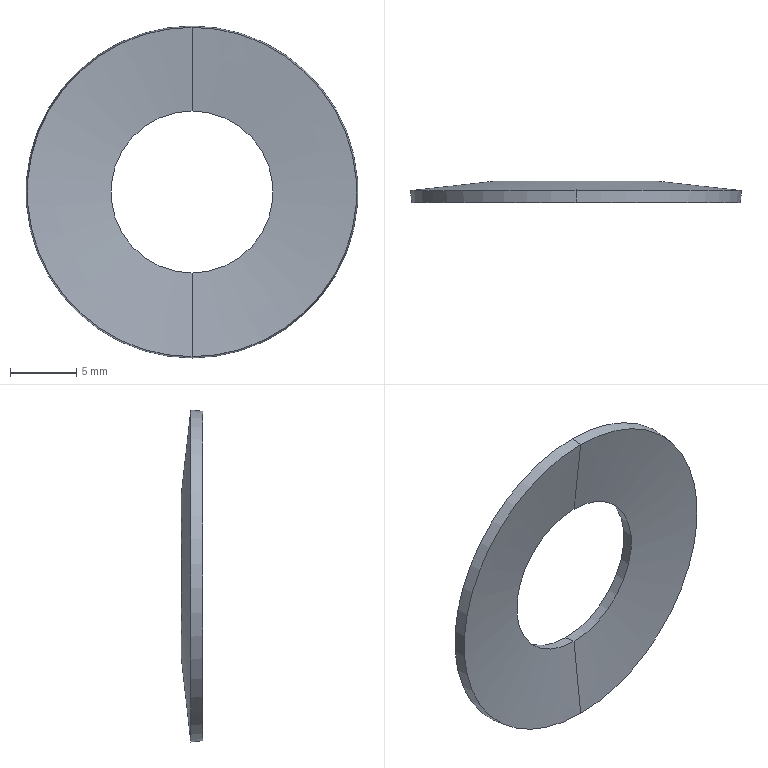Part | STEP file | 0228_001_SRBN25-A | 1 solid | 8 faces | box 25 x 1.6 x 25 mm | volume 333.381 mm3 | cone 8
STEP:
#1=CARTESIAN_POINT('',(0.,0.,0.));
#2=DIRECTION('',(0.,0.,1.));
#3=DIRECTION('',(1.,0.,0.));
#4=AXIS2_PLACEMENT_3D('',#1,#2,#3);
#5=CARTESIAN_POINT('',(0.,0.7,6.1));
#6=VERTEX_POINT('',#5);
#7=CARTESIAN_POINT('',(0.,1.594,6.2));
#8=VERTEX_POINT('',#7);
#9=CARTESIAN_POINT('',(0.,0.7,6.1));
#10=DIRECTION('',(0.,0.9938,0.1113));
#11=VECTOR('',#10,1.);
#12=LINE('',#9,#11);
#13=CARTESIAN_POINT('',(0.,0.7,0.));
#14=DIRECTION('',(0.,1.,0.));
#15=DIRECTION('',(0.,0.,1.));
#16=AXIS2_PLACEMENT_3D('',#13,#14,#15);
#17=CONICAL_SURFACE('',#16,6.1,0.1115);
#18=CARTESIAN_POINT('',(6.283,0.));
#19=DIRECTION('',(0.,1.));
#20=VECTOR('',#19,1.);
#21=LINE('',#18,#20);
#22=(GEOMETRIC_REPRESENTATION_CONTEXT(2)PARAMETRIC_REPRESENTATION_CONTEXT()REPRESENTATION_CONTEXT('',''));
#23=DEFINITIONAL_REPRESENTATION('',(#21),#22);
#24=PCURVE('',#17,#23);
#25=CARTESIAN_POINT('',(0.,0.7,0.));
#26=DIRECTION('',(0.,1.,0.));
#27=DIRECTION('',(0.,0.,1.));
#28=AXIS2_PLACEMENT_3D('',#25,#26,#27);
#29=CONICAL_SURFACE('',#28,6.1,0.1115);
#30=CARTESIAN_POINT('',(0.,0.));
#31=DIRECTION('',(0.,1.));
#32=VECTOR('',#31,1.);
#33=LINE('',#30,#32);
#34=(GEOMETRIC_REPRESENTATION_CONTEXT(2)PARAMETRIC_REPRESENTATION_CONTEXT()REPRESENTATION_CONTEXT('',''));
#35=DEFINITIONAL_REPRESENTATION('',(#33),#34);
#36=PCURVE('',#29,#35);
#37=SURFACE_CURVE('',#12,(#24,#36),.PCURVE_S1.);
#38=EDGE_CURVE('',#6,#8,#37,.T.);
#39=ORIENTED_EDGE('',*,*,#38,.T.);
#40=CARTESIAN_POINT('',(0.,1.594,-6.2));
#41=VERTEX_POINT('',#40);
#42=CARTESIAN_POINT('',(0.,1.594,0.));
#43=DIRECTION('',(0.,1.,0.));
#44=DIRECTION('',(0.,0.,1.));
#45=AXIS2_PLACEMENT_3D('',#42,#43,#44);
#46=CIRCLE('',#45,6.2);
#47=CARTESIAN_POINT('',(0.,0.8944));
#48=DIRECTION('',(1.,0.));
#49=VECTOR('',#48,1.);
#50=LINE('',#47,#49);
#51=(GEOMETRIC_REPRESENTATION_CONTEXT(2)PARAMETRIC_REPRESENTATION_CONTEXT()REPRESENTATION_CONTEXT('',''));
#52=DEFINITIONAL_REPRESENTATION('',(#50),#51);
#53=PCURVE('',#17,#52);
#54=CARTESIAN_POINT('',(0.,1.594,0.));
#55=DIRECTION('',(0.,-1.,0.));
#56=DIRECTION('',(0.,0.,-1.));
#57=AXIS2_PLACEMENT_3D('',#54,#55,#56);
#58=CONICAL_SURFACE('',#57,6.2,1.459);
#59=CARTESIAN_POINT('',(9.425,0.));
#60=DIRECTION('',(-1.,0.));
#61=VECTOR('',#60,1.);
#62=LINE('',#59,#61);
#63=(GEOMETRIC_REPRESENTATION_CONTEXT(2)PARAMETRIC_REPRESENTATION_CONTEXT()REPRESENTATION_CONTEXT('',''));
#64=DEFINITIONAL_REPRESENTATION('',(#62),#63);
#65=PCURVE('',#58,#64);
#66=SURFACE_CURVE('',#46,(#53,#65),.PCURVE_S1.);
#67=EDGE_CURVE('',#41,#8,#66,.T.);
#68=ORIENTED_EDGE('',*,*,#67,.F.);
#69=CARTESIAN_POINT('',(0.,0.7,-6.1));
#70=VERTEX_POINT('',#69);
#71=CARTESIAN_POINT('',(0.,0.7,-6.1));
#72=DIRECTION('',(0.,0.9938,-0.1113));
#73=VECTOR('',#72,1.);
#74=LINE('',#71,#73);
#75=CARTESIAN_POINT('',(3.142,0.));
#76=DIRECTION('',(0.,1.));
#77=VECTOR('',#76,1.);
#78=LINE('',#75,#77);
#79=(GEOMETRIC_REPRESENTATION_CONTEXT(2)PARAMETRIC_REPRESENTATION_CONTEXT()REPRESENTATION_CONTEXT('',''));
#80=DEFINITIONAL_REPRESENTATION('',(#78),#79);
#81=PCURVE('',#17,#80);
#82=CARTESIAN_POINT('',(3.142,0.));
#83=DIRECTION('',(0.,1.));
#84=VECTOR('',#83,1.);
#85=LINE('',#82,#84);
#86=(GEOMETRIC_REPRESENTATION_CONTEXT(2)PARAMETRIC_REPRESENTATION_CONTEXT()REPRESENTATION_CONTEXT('',''));
#87=DEFINITIONAL_REPRESENTATION('',(#85),#86);
#88=PCURVE('',#29,#87);
#89=SURFACE_CURVE('',#74,(#81,#88),.PCURVE_S1.);
#90=EDGE_CURVE('',#70,#41,#89,.T.);
#91=ORIENTED_EDGE('',*,*,#90,.F.);
#92=CARTESIAN_POINT('',(0.,0.7,0.));
#93=DIRECTION('',(0.,1.,0.));
#94=DIRECTION('',(0.,0.,1.));
#95=AXIS2_PLACEMENT_3D('',#92,#93,#94);
#96=CIRCLE('',#95,6.1);
#97=CARTESIAN_POINT('',(0.,0.));
#98=DIRECTION('',(1.,0.));
#99=VECTOR('',#98,1.);
#100=LINE('',#97,#99);
#101=(GEOMETRIC_REPRESENTATION_CONTEXT(2)PARAMETRIC_REPRESENTATION_CONTEXT()REPRESENTATION_CONTEXT('',''));
#102=DEFINITIONAL_REPRESENTATION('',(#100),#101);
#103=PCURVE('',#17,#102);
#104=CARTESIAN_POINT('',(0.,-0.005592,0.));
#105=DIRECTION('',(0.,-1.,0.));
#106=DIRECTION('',(0.,0.,-1.));
#107=AXIS2_PLACEMENT_3D('',#104,#105,#106);
#108=CONICAL_SURFACE('',#107,12.4,1.459);
#109=CARTESIAN_POINT('',(9.425,-0.7056));
#110=DIRECTION('',(-1.,0.));
#111=VECTOR('',#110,1.);
#112=LINE('',#109,#111);
#113=(GEOMETRIC_REPRESENTATION_CONTEXT(2)PARAMETRIC_REPRESENTATION_CONTEXT()REPRESENTATION_CONTEXT('',''));
#114=DEFINITIONAL_REPRESENTATION('',(#112),#113);
#115=PCURVE('',#108,#114);
#116=SURFACE_CURVE('',#96,(#103,#115),.PCURVE_S1.);
#117=EDGE_CURVE('',#70,#6,#116,.T.);
#118=ORIENTED_EDGE('',*,*,#117,.T.);
#119=EDGE_LOOP('',(#39,#68,#91,#118));
#120=FACE_BOUND('',#119,.F.);
#121=ADVANCED_FACE('',(#120),#17,.F.);
#122=CARTESIAN_POINT('',(0.,-0.005592,-12.4));
#123=VERTEX_POINT('',#122);
#124=CARTESIAN_POINT('',(0.,-0.005592,-12.4));
#125=DIRECTION('',(0.,-0.1113,-0.9938));
#126=VECTOR('',#125,1.);
#127=LINE('',#124,#126);
#128=CARTESIAN_POINT('',(6.283,0.));
#129=DIRECTION('',(0.,1.));
#130=VECTOR('',#129,1.);
#131=LINE('',#128,#130);
#132=(GEOMETRIC_REPRESENTATION_CONTEXT(2)PARAMETRIC_REPRESENTATION_CONTEXT()REPRESENTATION_CONTEXT('',''));
#133=DEFINITIONAL_REPRESENTATION('',(#131),#132);
#134=PCURVE('',#108,#133);
#135=CARTESIAN_POINT('',(0.,-0.005592,0.));
#136=DIRECTION('',(0.,-1.,0.));
#137=DIRECTION('',(0.,0.,-1.));
#138=AXIS2_PLACEMENT_3D('',#135,#136,#137);
#139=CONICAL_SURFACE('',#138,12.4,1.459);
#140=CARTESIAN_POINT('',(0.,0.));
#141=DIRECTION('',(0.,1.));
#142=VECTOR('',#141,1.);
#143=LINE('',#140,#142);
#144=(GEOMETRIC_REPRESENTATION_CONTEXT(2)PARAMETRIC_REPRESENTATION_CONTEXT()REPRESENTATION_CONTEXT('',''));
#145=DEFINITIONAL_REPRESENTATION('',(#143),#144);
#146=PCURVE('',#139,#145);
#147=SURFACE_CURVE('',#127,(#134,#146),.PCURVE_S1.);
#148=EDGE_CURVE('',#70,#123,#147,.T.);
#149=ORIENTED_EDGE('',*,*,#148,.T.);
#150=CARTESIAN_POINT('',(0.,-0.005592,12.4));
#151=VERTEX_POINT('',#150);
#152=CARTESIAN_POINT('',(0.,-0.005592,0.));
#153=DIRECTION('',(0.,1.,0.));
#154=DIRECTION('',(0.,0.,1.));
#155=AXIS2_PLACEMENT_3D('',#152,#153,#154);
#156=CIRCLE('',#155,12.4);
#157=CARTESIAN_POINT('',(9.425,0.));
#158=DIRECTION('',(-1.,0.));
#159=VECTOR('',#158,1.);
#160=LINE('',#157,#159);
#161=(GEOMETRIC_REPRESENTATION_CONTEXT(2)PARAMETRIC_REPRESENTATION_CONTEXT()REPRESENTATION_CONTEXT('',''));
#162=DEFINITIONAL_REPRESENTATION('',(#160),#161);
#163=PCURVE('',#108,#162);
#164=CARTESIAN_POINT('',(0.,0.8888,0.));
#165=DIRECTION('',(0.,1.,0.));
#166=DIRECTION('',(0.,0.,1.));
#167=AXIS2_PLACEMENT_3D('',#164,#165,#166);
#168=CONICAL_SURFACE('',#167,12.5,0.1115);
#169=CARTESIAN_POINT('',(0.,-0.8944));
#170=DIRECTION('',(1.,0.));
#171=VECTOR('',#170,1.);
#172=LINE('',#169,#171);
#173=(GEOMETRIC_REPRESENTATION_CONTEXT(2)PARAMETRIC_REPRESENTATION_CONTEXT()REPRESENTATION_CONTEXT('',''));
#174=DEFINITIONAL_REPRESENTATION('',(#172),#173);
#175=PCURVE('',#168,#174);
#176=SURFACE_CURVE('',#156,(#163,#175),.PCURVE_S1.);
#177=EDGE_CURVE('',#123,#151,#176,.T.);
#178=ORIENTED_EDGE('',*,*,#177,.T.);
#179=CARTESIAN_POINT('',(0.,-0.005592,12.4));
#180=DIRECTION('',(0.,-0.1113,0.9938));
#181=VECTOR('',#180,1.);
#182=LINE('',#179,#181);
#183=CARTESIAN_POINT('',(3.142,0.));
#184=DIRECTION('',(0.,1.));
#185=VECTOR('',#184,1.);
#186=LINE('',#183,#185);
#187=(GEOMETRIC_REPRESENTATION_CONTEXT(2)PARAMETRIC_REPRESENTATION_CONTEXT()REPRESENTATION_CONTEXT('',''));
#188=DEFINITIONAL_REPRESENTATION('',(#186),#187);
#189=PCURVE('',#108,#188);
#190=CARTESIAN_POINT('',(3.142,0.));
#191=DIRECTION('',(0.,1.));
#192=VECTOR('',#191,1.);
#193=LINE('',#190,#192);
#194=(GEOMETRIC_REPRESENTATION_CONTEXT(2)PARAMETRIC_REPRESENTATION_CONTEXT()REPRESENTATION_CONTEXT('',''));
#195=DEFINITIONAL_REPRESENTATION('',(#193),#194);
#196=PCURVE('',#139,#195);
#197=SURFACE_CURVE('',#182,(#189,#196),.PCURVE_S1.);
#198=EDGE_CURVE('',#6,#151,#197,.T.);
#199=ORIENTED_EDGE('',*,*,#198,.F.);
#200=ORIENTED_EDGE('',*,*,#117,.F.);
#201=EDGE_LOOP('',(#149,#178,#199,#200));
#202=FACE_BOUND('',#201,.F.);
#203=ADVANCED_FACE('',(#202),#108,.F.);
#204=CARTESIAN_POINT('',(0.,-0.005592,0.));
#205=DIRECTION('',(0.,1.,0.));
#206=DIRECTION('',(0.,0.,1.));
#207=AXIS2_PLACEMENT_3D('',#204,#205,#206);
#208=CIRCLE('',#207,12.4);
#209=CARTESIAN_POINT('',(0.,0.8888,0.));
#210=DIRECTION('',(0.,1.,0.));
#211=DIRECTION('',(0.,0.,1.));
#212=AXIS2_PLACEMENT_3D('',#209,#210,#211);
#213=CONICAL_SURFACE('',#212,12.5,0.1115);
#214=CARTESIAN_POINT('',(0.,-0.8944));
#215=DIRECTION('',(1.,0.));
#216=VECTOR('',#215,1.);
#217=LINE('',#214,#216);
#218=(GEOMETRIC_REPRESENTATION_CONTEXT(2)PARAMETRIC_REPRESENTATION_CONTEXT()REPRESENTATION_CONTEXT('',''));
#219=DEFINITIONAL_REPRESENTATION('',(#217),#218);
#220=PCURVE('',#213,#219);
#221=CARTESIAN_POINT('',(3.142,0.));
#222=DIRECTION('',(-1.,0.));
#223=VECTOR('',#222,1.);
#224=LINE('',#221,#223);
#225=(GEOMETRIC_REPRESENTATION_CONTEXT(2)PARAMETRIC_REPRESENTATION_CONTEXT()REPRESENTATION_CONTEXT('',''));
#226=DEFINITIONAL_REPRESENTATION('',(#224),#225);
#227=PCURVE('',#139,#226);
#228=SURFACE_CURVE('',#208,(#220,#227),.PCURVE_S1.);
#229=EDGE_CURVE('',#151,#123,#228,.T.);
#230=ORIENTED_EDGE('',*,*,#229,.T.);
#231=CARTESIAN_POINT('',(0.,0.8888,-12.5));
#232=VERTEX_POINT('',#231);
#233=CARTESIAN_POINT('',(0.,0.8888,-12.5));
#234=DIRECTION('',(0.,0.9938,-0.1113));
#235=VECTOR('',#234,1.);
#236=LINE('',#233,#235);
#237=CARTESIAN_POINT('',(3.142,0.));
#238=DIRECTION('',(0.,1.));
#239=VECTOR('',#238,1.);
#240=LINE('',#237,#239);
#241=(GEOMETRIC_REPRESENTATION_CONTEXT(2)PARAMETRIC_REPRESENTATION_CONTEXT()REPRESENTATION_CONTEXT('',''));
#242=DEFINITIONAL_REPRESENTATION('',(#240),#241);
#243=PCURVE('',#213,#242);
#244=CARTESIAN_POINT('',(3.142,0.));
#245=DIRECTION('',(0.,1.));
#246=VECTOR('',#245,1.);
#247=LINE('',#244,#246);
#248=(GEOMETRIC_REPRESENTATION_CONTEXT(2)PARAMETRIC_REPRESENTATION_CONTEXT()REPRESENTATION_CONTEXT('',''));
#249=DEFINITIONAL_REPRESENTATION('',(#247),#248);
#250=PCURVE('',#168,#249);
#251=SURFACE_CURVE('',#236,(#243,#250),.PCURVE_S1.);
#252=EDGE_CURVE('',#123,#232,#251,.T.);
#253=ORIENTED_EDGE('',*,*,#252,.T.);
#254=CARTESIAN_POINT('',(0.,0.8888,12.5));
#255=VERTEX_POINT('',#254);
#256=CARTESIAN_POINT('',(0.,0.8888,0.));
#257=DIRECTION('',(0.,1.,0.));
#258=DIRECTION('',(0.,0.,1.));
#259=AXIS2_PLACEMENT_3D('',#256,#257,#258);
#260=CIRCLE('',#259,12.5);
#261=CARTESIAN_POINT('',(0.,0.));
#262=DIRECTION('',(1.,0.));
#263=VECTOR('',#262,1.);
#264=LINE('',#261,#263);
#265=(GEOMETRIC_REPRESENTATION_CONTEXT(2)PARAMETRIC_REPRESENTATION_CONTEXT()REPRESENTATION_CONTEXT('',''));
#266=DEFINITIONAL_REPRESENTATION('',(#264),#265);
#267=PCURVE('',#213,#266);
#268=CARTESIAN_POINT('',(0.,1.594,0.));
#269=DIRECTION('',(0.,-1.,0.));
#270=DIRECTION('',(0.,0.,-1.));
#271=AXIS2_PLACEMENT_3D('',#268,#269,#270);
#272=CONICAL_SURFACE('',#271,6.2,1.459);
#273=CARTESIAN_POINT('',(3.142,0.7056));
#274=DIRECTION('',(-1.,0.));
#275=VECTOR('',#274,1.);
#276=LINE('',#273,#275);
#277=(GEOMETRIC_REPRESENTATION_CONTEXT(2)PARAMETRIC_REPRESENTATION_CONTEXT()REPRESENTATION_CONTEXT('',''));
#278=DEFINITIONAL_REPRESENTATION('',(#276),#277);
#279=PCURVE('',#272,#278);
#280=SURFACE_CURVE('',#260,(#267,#279),.PCURVE_S1.);
#281=EDGE_CURVE('',#255,#232,#280,.T.);
#282=ORIENTED_EDGE('',*,*,#281,.F.);
#283=CARTESIAN_POINT('',(0.,0.8888,12.5));
#284=DIRECTION('',(0.,0.9938,0.1113));
#285=VECTOR('',#284,1.);
#286=LINE('',#283,#285);
#287=CARTESIAN_POINT('',(0.,0.));
#288=DIRECTION('',(0.,1.));
#289=VECTOR('',#288,1.);
#290=LINE('',#287,#289);
#291=(GEOMETRIC_REPRESENTATION_CONTEXT(2)PARAMETRIC_REPRESENTATION_CONTEXT()REPRESENTATION_CONTEXT('',''));
#292=DEFINITIONAL_REPRESENTATION('',(#290),#291);
#293=PCURVE('',#213,#292);
#294=CARTESIAN_POINT('',(6.283,0.));
#295=DIRECTION('',(0.,1.));
#296=VECTOR('',#295,1.);
#297=LINE('',#294,#296);
#298=(GEOMETRIC_REPRESENTATION_CONTEXT(2)PARAMETRIC_REPRESENTATION_CONTEXT()REPRESENTATION_CONTEXT('',''));
#299=DEFINITIONAL_REPRESENTATION('',(#297),#298);
#300=PCURVE('',#168,#299);
#301=SURFACE_CURVE('',#286,(#293,#300),.PCURVE_S1.);
#302=EDGE_CURVE('',#151,#255,#301,.T.);
#303=ORIENTED_EDGE('',*,*,#302,.F.);
#304=EDGE_LOOP('',(#230,#253,#282,#303));
#305=FACE_BOUND('',#304,.T.);
#306=ADVANCED_FACE('',(#305),#213,.T.);
#307=CARTESIAN_POINT('',(0.,1.594,0.));
#308=DIRECTION('',(0.,1.,0.));
#309=DIRECTION('',(0.,0.,1.));
#310=AXIS2_PLACEMENT_3D('',#307,#308,#309);
#311=CIRCLE('',#310,6.2);
#312=CARTESIAN_POINT('',(3.142,0.));
#313=DIRECTION('',(-1.,0.));
#314=VECTOR('',#313,1.);
#315=LINE('',#312,#314);
#316=(GEOMETRIC_REPRESENTATION_CONTEXT(2)PARAMETRIC_REPRESENTATION_CONTEXT()REPRESENTATION_CONTEXT('',''));
#317=DEFINITIONAL_REPRESENTATION('',(#315),#316);
#318=PCURVE('',#272,#317);
#319=CARTESIAN_POINT('',(0.,0.8944));
#320=DIRECTION('',(1.,0.));
#321=VECTOR('',#320,1.);
#322=LINE('',#319,#321);
#323=(GEOMETRIC_REPRESENTATION_CONTEXT(2)PARAMETRIC_REPRESENTATION_CONTEXT()REPRESENTATION_CONTEXT('',''));
#324=DEFINITIONAL_REPRESENTATION('',(#322),#323);
#325=PCURVE('',#29,#324);
#326=SURFACE_CURVE('',#311,(#318,#325),.PCURVE_S1.);
#327=EDGE_CURVE('',#8,#41,#326,.T.);
#328=ORIENTED_EDGE('',*,*,#327,.F.);
#329=CARTESIAN_POINT('',(0.,1.594,6.2));
#330=DIRECTION('',(0.,-0.1113,0.9938));
#331=VECTOR('',#330,1.);
#332=LINE('',#329,#331);
#333=CARTESIAN_POINT('',(3.142,0.));
#334=DIRECTION('',(0.,1.));
#335=VECTOR('',#334,1.);
#336=LINE('',#333,#335);
#337=(GEOMETRIC_REPRESENTATION_CONTEXT(2)PARAMETRIC_REPRESENTATION_CONTEXT()REPRESENTATION_CONTEXT('',''));
#338=DEFINITIONAL_REPRESENTATION('',(#336),#337);
#339=PCURVE('',#272,#338);
#340=CARTESIAN_POINT('',(3.142,0.));
#341=DIRECTION('',(0.,1.));
#342=VECTOR('',#341,1.);
#343=LINE('',#340,#342);
#344=(GEOMETRIC_REPRESENTATION_CONTEXT(2)PARAMETRIC_REPRESENTATION_CONTEXT()REPRESENTATION_CONTEXT('',''));
#345=DEFINITIONAL_REPRESENTATION('',(#343),#344);
#346=PCURVE('',#58,#345);
#347=SURFACE_CURVE('',#332,(#339,#346),.PCURVE_S1.);
#348=EDGE_CURVE('',#8,#255,#347,.T.);
#349=ORIENTED_EDGE('',*,*,#348,.T.);
#350=ORIENTED_EDGE('',*,*,#281,.T.);
#351=CARTESIAN_POINT('',(0.,1.594,-6.2));
#352=DIRECTION('',(0.,-0.1113,-0.9938));
#353=VECTOR('',#352,1.);
#354=LINE('',#351,#353);
#355=CARTESIAN_POINT('',(0.,0.));
#356=DIRECTION('',(0.,1.));
#357=VECTOR('',#356,1.);
#358=LINE('',#355,#357);
#359=(GEOMETRIC_REPRESENTATION_CONTEXT(2)PARAMETRIC_REPRESENTATION_CONTEXT()REPRESENTATION_CONTEXT('',''));
#360=DEFINITIONAL_REPRESENTATION('',(#358),#359);
#361=PCURVE('',#272,#360);
#362=CARTESIAN_POINT('',(6.283,0.));
#363=DIRECTION('',(0.,1.));
#364=VECTOR('',#363,1.);
#365=LINE('',#362,#364);
#366=(GEOMETRIC_REPRESENTATION_CONTEXT(2)PARAMETRIC_REPRESENTATION_CONTEXT()REPRESENTATION_CONTEXT('',''));
#367=DEFINITIONAL_REPRESENTATION('',(#365),#366);
#368=PCURVE('',#58,#367);
#369=SURFACE_CURVE('',#354,(#361,#368),.PCURVE_S1.);
#370=EDGE_CURVE('',#41,#232,#369,.T.);
#371=ORIENTED_EDGE('',*,*,#370,.F.);
#372=EDGE_LOOP('',(#328,#349,#350,#371));
#373=FACE_BOUND('',#372,.T.);
#374=ADVANCED_FACE('',(#373),#272,.T.);
#375=ORIENTED_EDGE('',*,*,#348,.F.);
#376=ORIENTED_EDGE('',*,*,#67,.F.);
#377=ORIENTED_EDGE('',*,*,#370,.T.);
#378=CARTESIAN_POINT('',(0.,0.8888,0.));
#379=DIRECTION('',(0.,1.,0.));
#380=DIRECTION('',(0.,0.,1.));
#381=AXIS2_PLACEMENT_3D('',#378,#379,#380);
#382=CIRCLE('',#381,12.5);
#383=CARTESIAN_POINT('',(9.425,0.7056));
#384=DIRECTION('',(-1.,0.));
#385=VECTOR('',#384,1.);
#386=LINE('',#383,#385);
#387=(GEOMETRIC_REPRESENTATION_CONTEXT(2)PARAMETRIC_REPRESENTATION_CONTEXT()REPRESENTATION_CONTEXT('',''));
#388=DEFINITIONAL_REPRESENTATION('',(#386),#387);
#389=PCURVE('',#58,#388);
#390=CARTESIAN_POINT('',(0.,0.));
#391=DIRECTION('',(1.,0.));
#392=VECTOR('',#391,1.);
#393=LINE('',#390,#392);
#394=(GEOMETRIC_REPRESENTATION_CONTEXT(2)PARAMETRIC_REPRESENTATION_CONTEXT()REPRESENTATION_CONTEXT('',''));
#395=DEFINITIONAL_REPRESENTATION('',(#393),#394);
#396=PCURVE('',#168,#395);
#397=SURFACE_CURVE('',#382,(#389,#396),.PCURVE_S1.);
#398=EDGE_CURVE('',#232,#255,#397,.T.);
#399=ORIENTED_EDGE('',*,*,#398,.T.);
#400=EDGE_LOOP('',(#375,#376,#377,#399));
#401=FACE_BOUND('',#400,.T.);
#402=ADVANCED_FACE('',(#401),#58,.T.);
#403=ORIENTED_EDGE('',*,*,#252,.F.);
#404=ORIENTED_EDGE('',*,*,#177,.T.);
#405=ORIENTED_EDGE('',*,*,#302,.T.);
#406=ORIENTED_EDGE('',*,*,#398,.F.);
#407=EDGE_LOOP('',(#403,#404,#405,#406));
#408=FACE_BOUND('',#407,.T.);
#409=ADVANCED_FACE('',(#408),#168,.T.);
#410=ORIENTED_EDGE('',*,*,#229,.T.);
#411=ORIENTED_EDGE('',*,*,#148,.F.);
#412=CARTESIAN_POINT('',(0.,0.7,0.));
#413=DIRECTION('',(0.,1.,0.));
#414=DIRECTION('',(0.,0.,1.));
#415=AXIS2_PLACEMENT_3D('',#412,#413,#414);
#416=CIRCLE('',#415,6.1);
#417=CARTESIAN_POINT('',(3.142,-0.7056));
#418=DIRECTION('',(-1.,0.));
#419=VECTOR('',#418,1.);
#420=LINE('',#417,#419);
#421=(GEOMETRIC_REPRESENTATION_CONTEXT(2)PARAMETRIC_REPRESENTATION_CONTEXT()REPRESENTATION_CONTEXT('',''));
#422=DEFINITIONAL_REPRESENTATION('',(#420),#421);
#423=PCURVE('',#139,#422);
#424=CARTESIAN_POINT('',(0.,0.));
#425=DIRECTION('',(1.,0.));
#426=VECTOR('',#425,1.);
#427=LINE('',#424,#426);
#428=(GEOMETRIC_REPRESENTATION_CONTEXT(2)PARAMETRIC_REPRESENTATION_CONTEXT()REPRESENTATION_CONTEXT('',''));
#429=DEFINITIONAL_REPRESENTATION('',(#427),#428);
#430=PCURVE('',#29,#429);
#431=SURFACE_CURVE('',#416,(#423,#430),.PCURVE_S1.);
#432=EDGE_CURVE('',#6,#70,#431,.T.);
#433=ORIENTED_EDGE('',*,*,#432,.F.);
#434=ORIENTED_EDGE('',*,*,#198,.T.);
#435=EDGE_LOOP('',(#410,#411,#433,#434));
#436=FACE_BOUND('',#435,.F.);
#437=ADVANCED_FACE('',(#436),#139,.F.);
#438=ORIENTED_EDGE('',*,*,#327,.F.);
#439=ORIENTED_EDGE('',*,*,#38,.F.);
#440=ORIENTED_EDGE('',*,*,#432,.T.);
#441=ORIENTED_EDGE('',*,*,#90,.T.);
#442=EDGE_LOOP('',(#438,#439,#440,#441));
#443=FACE_BOUND('',#442,.F.);
#444=ADVANCED_FACE('',(#443),#29,.F.);
#445=CLOSED_SHELL('',(#121,#203,#306,#374,#402,#409,#437,#444));
#446=MANIFOLD_SOLID_BREP('',#445);
#447=(LENGTH_UNIT()NAMED_UNIT(*)SI_UNIT(.MILLI.,.METRE.));
#448=UNCERTAINTY_MEASURE_WITH_UNIT(LENGTH_MEASURE(0.0000001),#447,'','');
#449=(NAMED_UNIT(*)PLANE_ANGLE_UNIT()SI_UNIT($,.RADIAN.));
#450=(NAMED_UNIT(*)SI_UNIT($,.STERADIAN.)SOLID_ANGLE_UNIT());
#451=(GEOMETRIC_REPRESENTATION_CONTEXT(3)GLOBAL_UNCERTAINTY_ASSIGNED_CONTEXT((#448))GLOBAL_UNIT_ASSIGNED_CONTEXT((#447,#449,#450))REPRESENTATION_CONTEXT('',''));
#452=ADVANCED_BREP_SHAPE_REPRESENTATION('',(#4,#446),#451);